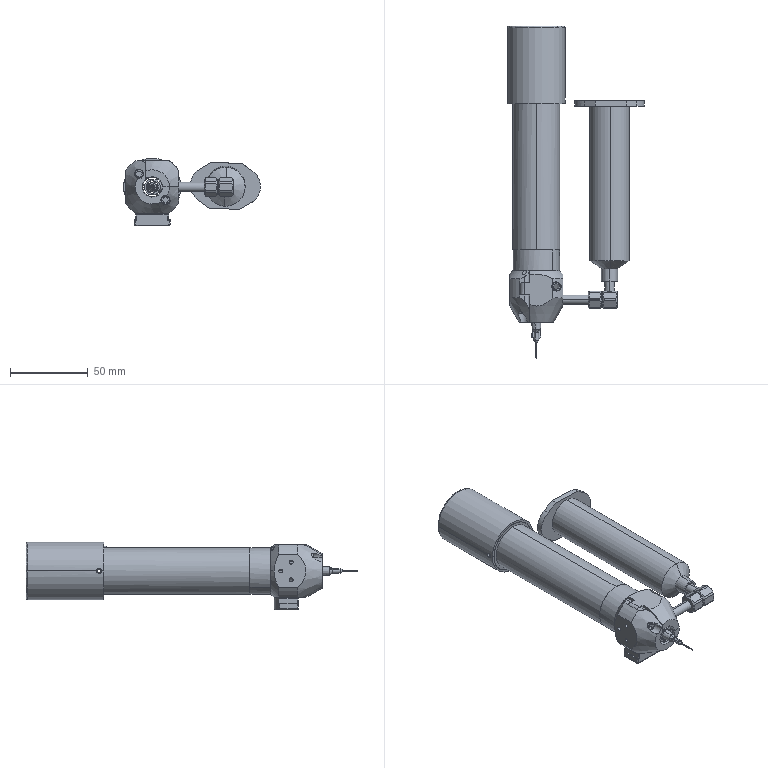Part | NX | features BREP 12 | 6 solids | 271 faces | box 88.087 x 213.5 x 43.5 mm | volume 197364 mm3 | cylinder 124 | plane 105 | cone 29 | torus 8 | spline 5 | commonest cylinder face diameters 6 x16 12 x16 1 x10 2.5 x10 8 x8 40 x6